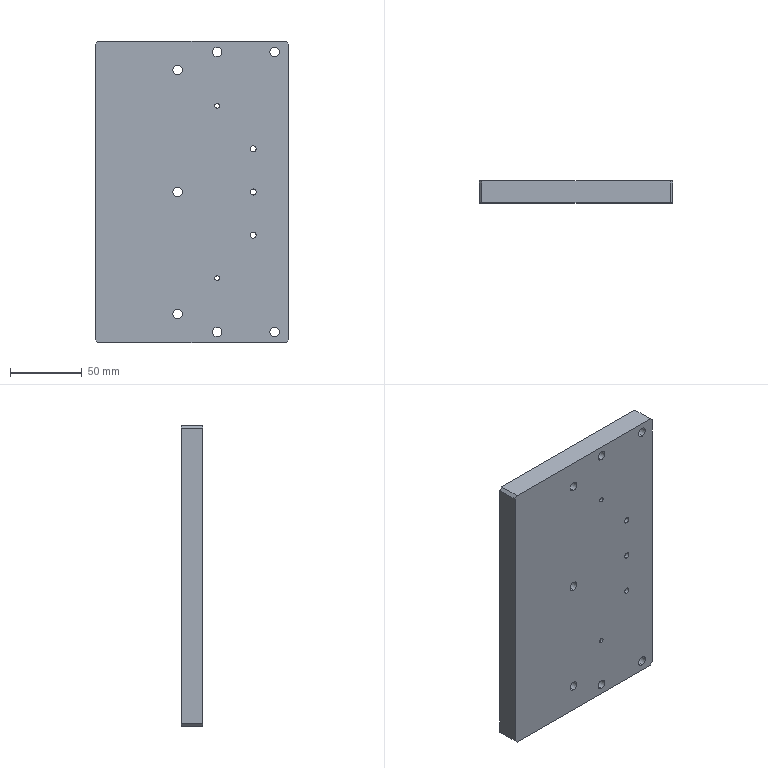Part | SolidWorks | features BaseBody 1 | 1 solid | 87 faces | box 135 x 15 x 210 mm | volume 416442 mm3 | cylinder 54 | plane 17 | cone 16 | commonest cylinder face diameters 3.3 x20 6.6 x14 11 x14 4.2 x6